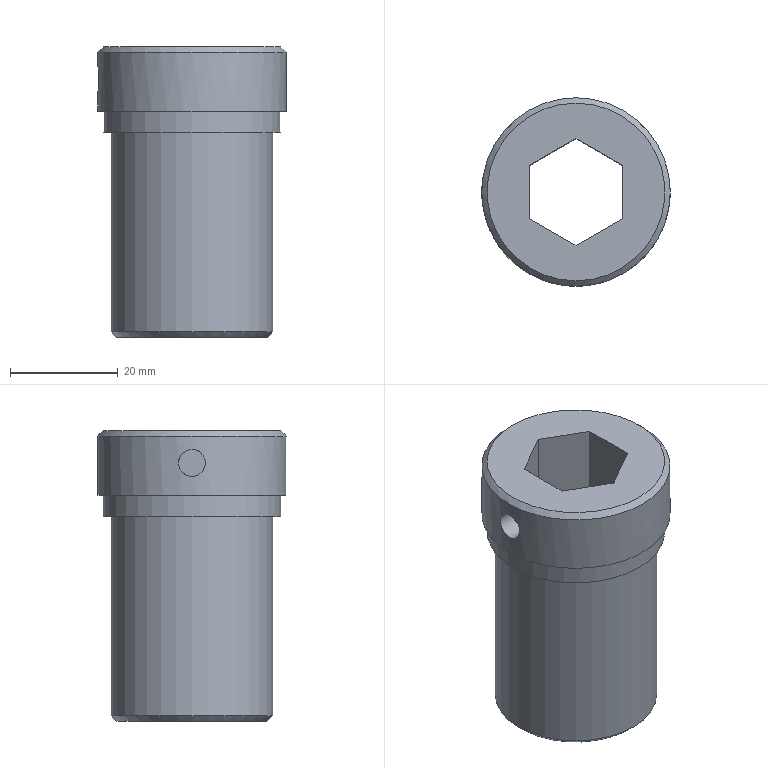Part | STEP file | JBJ-P-1002-08 | 1 solid | 16 faces | box 35 x 35 x 54 mm | volume 27719 mm3 | plane 10 | cylinder 4 | cone 2 | commonest cylinder face diameters 5 x1 30 x1 33 x1 35 x1
STEP:
#1=CARTESIAN_POINT('',(8.6,4.965,-54.));
#2=VERTEX_POINT('',#1);
#3=CARTESIAN_POINT('',(0.,9.93,-54.));
#4=VERTEX_POINT('',#3);
#5=CARTESIAN_POINT('',(8.6,4.965,-54.));
#6=DIRECTION('',(-0.866,0.5,0.));
#7=VECTOR('',#6,1000.);
#8=LINE('',#5,#7);
#9=EDGE_CURVE('',#2,#4,#8,.T.);
#10=ORIENTED_EDGE('',*,*,#9,.T.);
#11=CARTESIAN_POINT('',(-8.6,4.965,-54.));
#12=VERTEX_POINT('',#11);
#13=CARTESIAN_POINT('',(0.,9.93,-54.));
#14=DIRECTION('',(-0.866,-0.5,0.));
#15=VECTOR('',#14,1000.);
#16=LINE('',#13,#15);
#17=EDGE_CURVE('',#4,#12,#16,.T.);
#18=ORIENTED_EDGE('',*,*,#17,.T.);
#19=CARTESIAN_POINT('',(-8.6,-4.965,-54.));
#20=VERTEX_POINT('',#19);
#21=CARTESIAN_POINT('',(-8.6,4.965,-54.));
#22=DIRECTION('',(0.,-1.,0.));
#23=VECTOR('',#22,1000.);
#24=LINE('',#21,#23);
#25=EDGE_CURVE('',#12,#20,#24,.T.);
#26=ORIENTED_EDGE('',*,*,#25,.T.);
#27=CARTESIAN_POINT('',(0.,-9.93,-54.));
#28=VERTEX_POINT('',#27);
#29=CARTESIAN_POINT('',(-8.6,-4.965,-54.));
#30=DIRECTION('',(0.866,-0.5,0.));
#31=VECTOR('',#30,1000.);
#32=LINE('',#29,#31);
#33=EDGE_CURVE('',#20,#28,#32,.T.);
#34=ORIENTED_EDGE('',*,*,#33,.T.);
#35=CARTESIAN_POINT('',(8.6,-4.965,-54.));
#36=VERTEX_POINT('',#35);
#37=CARTESIAN_POINT('',(0.,-9.93,-54.));
#38=DIRECTION('',(0.866,0.5,0.));
#39=VECTOR('',#38,1000.);
#40=LINE('',#37,#39);
#41=EDGE_CURVE('',#28,#36,#40,.T.);
#42=ORIENTED_EDGE('',*,*,#41,.T.);
#43=CARTESIAN_POINT('',(8.6,-4.965,-54.));
#44=DIRECTION('',(0.,1.,0.));
#45=VECTOR('',#44,1000.);
#46=LINE('',#43,#45);
#47=EDGE_CURVE('',#36,#2,#46,.T.);
#48=ORIENTED_EDGE('',*,*,#47,.T.);
#49=EDGE_LOOP('',(#10,#18,#26,#34,#42,#48));
#50=FACE_BOUND('',#49,.T.);
#51=CARTESIAN_POINT('',(0.,14.,-54.));
#52=VERTEX_POINT('',#51);
#53=CARTESIAN_POINT('',(0.,0.,-54.));
#54=DIRECTION('',(0.,0.,-1.));
#55=DIRECTION('',(0.,1.,0.));
#56=AXIS2_PLACEMENT_3D('',#53,#54,#55);
#57=CIRCLE('',#56,14.);
#58=EDGE_CURVE('',#52,#52,#57,.T.);
#59=ORIENTED_EDGE('',*,*,#58,.T.);
#60=EDGE_LOOP('',(#59));
#61=FACE_OUTER_BOUND('',#60,.T.);
#62=CARTESIAN_POINT('',(0.,0.,-54.));
#63=DIRECTION('',(0.,0.,-1.));
#64=DIRECTION('',(0.,1.,0.));
#65=AXIS2_PLACEMENT_3D('',#62,#63,#64);
#66=PLANE('',#65);
#67=ADVANCED_FACE('',(#50,#61),#66,.T.);
#68=ORIENTED_EDGE('',*,*,#58,.F.);
#69=EDGE_LOOP('',(#68));
#70=FACE_BOUND('',#69,.T.);
#71=CARTESIAN_POINT('',(0.,15.,-53.));
#72=VERTEX_POINT('',#71);
#73=CARTESIAN_POINT('',(0.,0.,-53.));
#74=DIRECTION('',(0.,0.,-1.));
#75=DIRECTION('',(0.,1.,0.));
#76=AXIS2_PLACEMENT_3D('',#73,#74,#75);
#77=CIRCLE('',#76,15.);
#78=EDGE_CURVE('',#72,#72,#77,.T.);
#79=ORIENTED_EDGE('',*,*,#78,.T.);
#80=EDGE_LOOP('',(#79));
#81=FACE_OUTER_BOUND('',#80,.T.);
#82=CARTESIAN_POINT('',(0.,0.,-53.));
#83=DIRECTION('',(0.,0.,1.));
#84=DIRECTION('',(0.,-1.,0.));
#85=AXIS2_PLACEMENT_3D('',#82,#83,#84);
#86=CONICAL_SURFACE('',#85,15.,0.7854);
#87=ADVANCED_FACE('',(#70,#81),#86,.T.);
#88=ORIENTED_EDGE('',*,*,#78,.F.);
#89=EDGE_LOOP('',(#88));
#90=FACE_OUTER_BOUND('',#89,.T.);
#91=CARTESIAN_POINT('',(0.,15.,-16.));
#92=VERTEX_POINT('',#91);
#93=CARTESIAN_POINT('',(0.,0.,-16.));
#94=DIRECTION('',(0.,0.,-1.));
#95=DIRECTION('',(0.,1.,0.));
#96=AXIS2_PLACEMENT_3D('',#93,#94,#95);
#97=CIRCLE('',#96,15.);
#98=EDGE_CURVE('',#92,#92,#97,.T.);
#99=ORIENTED_EDGE('',*,*,#98,.T.);
#100=EDGE_LOOP('',(#99));
#101=FACE_OUTER_BOUND('',#100,.T.);
#102=CARTESIAN_POINT('',(0.,0.,-54.));
#103=DIRECTION('',(0.,0.,-1.));
#104=DIRECTION('',(0.,1.,0.));
#105=AXIS2_PLACEMENT_3D('',#102,#103,#104);
#106=CYLINDRICAL_SURFACE('',#105,15.);
#107=ADVANCED_FACE('',(#90,#101),#106,.T.);
#108=ORIENTED_EDGE('',*,*,#98,.F.);
#109=EDGE_LOOP('',(#108));
#110=FACE_BOUND('',#109,.T.);
#111=CARTESIAN_POINT('',(0.,16.5,-16.));
#112=VERTEX_POINT('',#111);
#113=CARTESIAN_POINT('',(0.,0.,-16.));
#114=DIRECTION('',(0.,0.,-1.));
#115=DIRECTION('',(0.,1.,0.));
#116=AXIS2_PLACEMENT_3D('',#113,#114,#115);
#117=CIRCLE('',#116,16.5);
#118=EDGE_CURVE('',#112,#112,#117,.T.);
#119=ORIENTED_EDGE('',*,*,#118,.T.);
#120=EDGE_LOOP('',(#119));
#121=FACE_OUTER_BOUND('',#120,.T.);
#122=CARTESIAN_POINT('',(0.,0.,-16.));
#123=DIRECTION('',(0.,0.,1.));
#124=DIRECTION('',(0.,-1.,0.));
#125=AXIS2_PLACEMENT_3D('',#122,#123,#124);
#126=PLANE('',#125);
#127=ADVANCED_FACE('',(#110,#121),#126,.F.);
#128=ORIENTED_EDGE('',*,*,#118,.F.);
#129=EDGE_LOOP('',(#128));
#130=FACE_OUTER_BOUND('',#129,.T.);
#131=CARTESIAN_POINT('',(0.,16.5,-12.));
#132=VERTEX_POINT('',#131);
#133=CARTESIAN_POINT('',(0.,0.,-12.));
#134=DIRECTION('',(0.,0.,-1.));
#135=DIRECTION('',(0.,1.,0.));
#136=AXIS2_PLACEMENT_3D('',#133,#134,#135);
#137=CIRCLE('',#136,16.5);
#138=EDGE_CURVE('',#132,#132,#137,.T.);
#139=ORIENTED_EDGE('',*,*,#138,.T.);
#140=EDGE_LOOP('',(#139));
#141=FACE_OUTER_BOUND('',#140,.T.);
#142=CARTESIAN_POINT('',(0.,0.,-54.));
#143=DIRECTION('',(0.,0.,-1.));
#144=DIRECTION('',(0.,1.,0.));
#145=AXIS2_PLACEMENT_3D('',#142,#143,#144);
#146=CYLINDRICAL_SURFACE('',#145,16.5);
#147=ADVANCED_FACE('',(#130,#141),#146,.T.);
#148=ORIENTED_EDGE('',*,*,#138,.F.);
#149=EDGE_LOOP('',(#148));
#150=FACE_BOUND('',#149,.T.);
#151=CARTESIAN_POINT('',(0.,17.5,-12.));
#152=VERTEX_POINT('',#151);
#153=CARTESIAN_POINT('',(0.,0.,-12.));
#154=DIRECTION('',(0.,0.,-1.));
#155=DIRECTION('',(0.,1.,0.));
#156=AXIS2_PLACEMENT_3D('',#153,#154,#155);
#157=CIRCLE('',#156,17.5);
#158=EDGE_CURVE('',#152,#152,#157,.T.);
#159=ORIENTED_EDGE('',*,*,#158,.T.);
#160=EDGE_LOOP('',(#159));
#161=FACE_OUTER_BOUND('',#160,.T.);
#162=CARTESIAN_POINT('',(0.,0.,-12.));
#163=DIRECTION('',(0.,0.,1.));
#164=DIRECTION('',(0.,-1.,0.));
#165=AXIS2_PLACEMENT_3D('',#162,#163,#164);
#166=PLANE('',#165);
#167=ADVANCED_FACE('',(#150,#161),#166,.F.);
#168=CARTESIAN_POINT('',(0.,-17.5,-1.));
#169=VERTEX_POINT('',#168);
#170=CARTESIAN_POINT('',(0.,0.,-1.));
#171=DIRECTION('',(0.,0.,-1.));
#172=DIRECTION('',(0.,-1.,0.));
#173=AXIS2_PLACEMENT_3D('',#170,#171,#172);
#174=CIRCLE('',#173,17.5);
#175=EDGE_CURVE('',#169,#169,#174,.T.);
#176=ORIENTED_EDGE('',*,*,#175,.T.);
#177=EDGE_LOOP('',(#176));
#178=FACE_OUTER_BOUND('',#177,.T.);
#179=CARTESIAN_POINT('',(-17.5,0.,-3.5));
#180=VERTEX_POINT('',#179);
#181=CARTESIAN_POINT('',(-17.5,0.,-3.5));
#182=CARTESIAN_POINT('',(-17.5,-0.1654,-3.5));
#183=CARTESIAN_POINT('',(-17.498,-0.328,-3.516));
#184=CARTESIAN_POINT('',(-17.489,-0.6478,-3.58));
#185=CARTESIAN_POINT('',(-17.482,-0.8067,-3.628));
#186=CARTESIAN_POINT('',(-17.465,-1.109,-3.754));
#187=CARTESIAN_POINT('',(-17.456,-1.253,-3.83));
#188=CARTESIAN_POINT('',(-17.434,-1.524,-4.012));
#189=CARTESIAN_POINT('',(-17.422,-1.653,-4.117));
#190=CARTESIAN_POINT('',(-17.399,-1.883,-4.348));
#191=CARTESIAN_POINT('',(-17.387,-1.987,-4.473));
#192=CARTESIAN_POINT('',(-17.365,-2.169,-4.747));
#193=CARTESIAN_POINT('',(-17.355,-2.247,-4.892));
#194=CARTESIAN_POINT('',(-17.339,-2.372,-5.192));
#195=CARTESIAN_POINT('',(-17.332,-2.42,-5.35));
#196=CARTESIAN_POINT('',(-17.323,-2.484,-5.673));
#197=CARTESIAN_POINT('',(-17.321,-2.5,-5.835));
#198=CARTESIAN_POINT('',(-17.32,-2.5,-6.162));
#199=CARTESIAN_POINT('',(-17.323,-2.484,-6.328));
#200=CARTESIAN_POINT('',(-17.332,-2.42,-6.649));
#201=CARTESIAN_POINT('',(-17.339,-2.373,-6.804));
#202=CARTESIAN_POINT('',(-17.355,-2.247,-7.107));
#203=CARTESIAN_POINT('',(-17.365,-2.169,-7.253));
#204=CARTESIAN_POINT('',(-17.387,-1.988,-7.524));
#205=CARTESIAN_POINT('',(-17.399,-1.885,-7.651));
#206=CARTESIAN_POINT('',(-17.422,-1.652,-7.884));
#207=CARTESIAN_POINT('',(-17.434,-1.526,-7.987));
#208=CARTESIAN_POINT('',(-17.455,-1.255,-8.168));
#209=CARTESIAN_POINT('',(-17.465,-1.109,-8.246));
#210=CARTESIAN_POINT('',(-17.482,-0.8066,-8.372));
#211=CARTESIAN_POINT('',(-17.489,-0.6508,-8.419));
#212=CARTESIAN_POINT('',(-17.498,-0.33,-8.484));
#213=CARTESIAN_POINT('',(-17.5,-0.1642,-8.5));
#214=CARTESIAN_POINT('',(-17.5,0.1623,-8.5));
#215=CARTESIAN_POINT('',(-17.498,0.3247,-8.484));
#216=CARTESIAN_POINT('',(-17.489,0.6478,-8.42));
#217=CARTESIAN_POINT('',(-17.482,0.8054,-8.372));
#218=CARTESIAN_POINT('',(-17.466,1.106,-8.248));
#219=CARTESIAN_POINT('',(-17.456,1.252,-8.17));
#220=CARTESIAN_POINT('',(-17.434,1.525,-7.988));
#221=CARTESIAN_POINT('',(-17.422,1.651,-7.885));
#222=CARTESIAN_POINT('',(-17.399,1.881,-7.654));
#223=CARTESIAN_POINT('',(-17.387,1.987,-7.526));
#224=CARTESIAN_POINT('',(-17.365,2.168,-7.255));
#225=CARTESIAN_POINT('',(-17.355,2.245,-7.111));
#226=CARTESIAN_POINT('',(-17.339,2.371,-6.809));
#227=CARTESIAN_POINT('',(-17.332,2.42,-6.65));
#228=CARTESIAN_POINT('',(-17.323,2.483,-6.33));
#229=CARTESIAN_POINT('',(-17.321,2.5,-6.167));
#230=CARTESIAN_POINT('',(-17.32,2.5,-5.837));
#231=CARTESIAN_POINT('',(-17.323,2.484,-5.674));
#232=CARTESIAN_POINT('',(-17.332,2.421,-5.354));
#233=CARTESIAN_POINT('',(-17.339,2.373,-5.195));
#234=CARTESIAN_POINT('',(-17.355,2.247,-4.893));
#235=CARTESIAN_POINT('',(-17.365,2.171,-4.749));
#236=CARTESIAN_POINT('',(-17.387,1.989,-4.477));
#237=CARTESIAN_POINT('',(-17.399,1.884,-4.349));
#238=CARTESIAN_POINT('',(-17.434,1.539,-4.003));
#239=CARTESIAN_POINT('',(-17.457,1.261,-3.817));
#240=CARTESIAN_POINT('',(-17.482,0.8097,-3.629));
#241=CARTESIAN_POINT('',(-17.489,0.6519,-3.581));
#242=CARTESIAN_POINT('',(-17.498,0.3288,-3.516));
#243=CARTESIAN_POINT('',(-17.5,0.1654,-3.5));
#244=CARTESIAN_POINT('',(-17.5,0.,-3.5));
#245=B_SPLINE_CURVE_WITH_KNOTS('',3,(#181,#182,#183,#184,#185,#186,#187,#188,#189,#190,#191,#192,#193,#194,#195,#196,#197,#198,#199,#200,#201,#202,#203,#204,#205,#206,#207,#208,#209,#210,#211,#212,#213,#214,#215,#216,#217,#218,#219,#220,#221,#222,#223,#224,#225,#226,#227,#228,#229,#230,#231,#232,#233,#234,#235,#236,#237,#238,#239,#240,#241,#242,#243,#244),.UNSPECIFIED.,.T.,.F.,(4,2,2,2,2,2,2,2,2,2,2,2,2,2,2,2,2,2,2,2,2,2,2,2,2,2,2,2,2,2,2,4),(0.,0.0004891,0.0009781,0.001467,0.001956,0.002445,0.002934,0.003424,0.003913,0.004402,0.004891,0.00538,0.005869,0.006358,0.006847,0.007336,0.007825,0.008314,0.008803,0.009292,0.009781,0.01027,0.01076,0.01125,0.01174,0.01223,0.01272,0.01321,0.01369,0.01467,0.01516,0.01565),.UNSPECIFIED.);
#246=EDGE_CURVE('',#180,#180,#245,.T.);
#247=ORIENTED_EDGE('',*,*,#246,.T.);
#248=EDGE_LOOP('',(#247));
#249=FACE_BOUND('',#248,.T.);
#250=ORIENTED_EDGE('',*,*,#158,.F.);
#251=EDGE_LOOP('',(#250));
#252=FACE_OUTER_BOUND('',#251,.T.);
#253=CARTESIAN_POINT('',(0.,0.,-54.));
#254=DIRECTION('',(0.,0.,-1.));
#255=DIRECTION('',(0.,1.,0.));
#256=AXIS2_PLACEMENT_3D('',#253,#254,#255);
#257=CYLINDRICAL_SURFACE('',#256,17.5);
#258=ADVANCED_FACE('',(#178,#249,#252),#257,.T.);
#259=CARTESIAN_POINT('',(0.,-16.5,0.));
#260=VERTEX_POINT('',#259);
#261=CARTESIAN_POINT('',(0.,0.,0.));
#262=DIRECTION('',(0.,0.,1.));
#263=DIRECTION('',(0.,-1.,0.));
#264=AXIS2_PLACEMENT_3D('',#261,#262,#263);
#265=CIRCLE('',#264,16.5);
#266=EDGE_CURVE('',#260,#260,#265,.T.);
#267=ORIENTED_EDGE('',*,*,#266,.T.);
#268=EDGE_LOOP('',(#267));
#269=FACE_OUTER_BOUND('',#268,.T.);
#270=CARTESIAN_POINT('',(8.6,4.965,0.));
#271=VERTEX_POINT('',#270);
#272=CARTESIAN_POINT('',(0.,9.93,0.));
#273=VERTEX_POINT('',#272);
#274=CARTESIAN_POINT('',(8.6,4.965,0.));
#275=DIRECTION('',(-0.866,0.5,0.));
#276=VECTOR('',#275,1000.);
#277=LINE('',#274,#276);
#278=EDGE_CURVE('',#271,#273,#277,.T.);
#279=ORIENTED_EDGE('',*,*,#278,.F.);
#280=CARTESIAN_POINT('',(8.6,-4.965,0.));
#281=VERTEX_POINT('',#280);
#282=CARTESIAN_POINT('',(8.6,-4.965,0.));
#283=DIRECTION('',(0.,1.,0.));
#284=VECTOR('',#283,1000.);
#285=LINE('',#282,#284);
#286=EDGE_CURVE('',#281,#271,#285,.T.);
#287=ORIENTED_EDGE('',*,*,#286,.F.);
#288=CARTESIAN_POINT('',(0.,-9.93,0.));
#289=VERTEX_POINT('',#288);
#290=CARTESIAN_POINT('',(0.,-9.93,0.));
#291=DIRECTION('',(0.866,0.5,0.));
#292=VECTOR('',#291,1000.);
#293=LINE('',#290,#292);
#294=EDGE_CURVE('',#289,#281,#293,.T.);
#295=ORIENTED_EDGE('',*,*,#294,.F.);
#296=CARTESIAN_POINT('',(-8.6,-4.965,0.));
#297=VERTEX_POINT('',#296);
#298=CARTESIAN_POINT('',(-8.6,-4.965,0.));
#299=DIRECTION('',(0.866,-0.5,0.));
#300=VECTOR('',#299,1000.);
#301=LINE('',#298,#300);
#302=EDGE_CURVE('',#297,#289,#301,.T.);
#303=ORIENTED_EDGE('',*,*,#302,.F.);
#304=CARTESIAN_POINT('',(-8.6,4.965,0.));
#305=VERTEX_POINT('',#304);
#306=CARTESIAN_POINT('',(-8.6,4.965,0.));
#307=DIRECTION('',(0.,-1.,0.));
#308=VECTOR('',#307,1000.);
#309=LINE('',#306,#308);
#310=EDGE_CURVE('',#305,#297,#309,.T.);
#311=ORIENTED_EDGE('',*,*,#310,.F.);
#312=CARTESIAN_POINT('',(0.,9.93,0.));
#313=DIRECTION('',(-0.866,-0.5,0.));
#314=VECTOR('',#313,1000.);
#315=LINE('',#312,#314);
#316=EDGE_CURVE('',#273,#305,#315,.T.);
#317=ORIENTED_EDGE('',*,*,#316,.F.);
#318=EDGE_LOOP('',(#279,#287,#295,#303,#311,#317));
#319=FACE_BOUND('',#318,.T.);
#320=CARTESIAN_POINT('',(0.,0.,0.));
#321=DIRECTION('',(0.,0.,1.));
#322=DIRECTION('',(0.,-1.,0.));
#323=AXIS2_PLACEMENT_3D('',#320,#321,#322);
#324=PLANE('',#323);
#325=ADVANCED_FACE('',(#269,#319),#324,.T.);
#326=ORIENTED_EDGE('',*,*,#278,.T.);
#327=CARTESIAN_POINT('',(0.,9.93,-54.));
#328=DIRECTION('',(0.,0.,1.));
#329=VECTOR('',#328,1000.);
#330=LINE('',#327,#329);
#331=EDGE_CURVE('',#4,#273,#330,.T.);
#332=ORIENTED_EDGE('',*,*,#331,.F.);
#333=ORIENTED_EDGE('',*,*,#9,.F.);
#334=CARTESIAN_POINT('',(8.6,4.965,-54.));
#335=DIRECTION('',(0.,0.,1.));
#336=VECTOR('',#335,1000.);
#337=LINE('',#334,#336);
#338=EDGE_CURVE('',#2,#271,#337,.T.);
#339=ORIENTED_EDGE('',*,*,#338,.T.);
#340=EDGE_LOOP('',(#326,#332,#333,#339));
#341=FACE_OUTER_BOUND('',#340,.T.);
#342=CARTESIAN_POINT('',(8.6,4.965,-54.));
#343=DIRECTION('',(0.5,0.866,0.));
#344=DIRECTION('',(-0.866,0.5,0.));
#345=AXIS2_PLACEMENT_3D('',#342,#343,#344);
#346=PLANE('',#345);
#347=ADVANCED_FACE('',(#341),#346,.F.);
#348=ORIENTED_EDGE('',*,*,#286,.T.);
#349=ORIENTED_EDGE('',*,*,#338,.F.);
#350=ORIENTED_EDGE('',*,*,#47,.F.);
#351=CARTESIAN_POINT('',(8.6,-4.965,-54.));
#352=DIRECTION('',(0.,0.,1.));
#353=VECTOR('',#352,1000.);
#354=LINE('',#351,#353);
#355=EDGE_CURVE('',#36,#281,#354,.T.);
#356=ORIENTED_EDGE('',*,*,#355,.T.);
#357=EDGE_LOOP('',(#348,#349,#350,#356));
#358=FACE_OUTER_BOUND('',#357,.T.);
#359=CARTESIAN_POINT('',(8.6,-4.965,-54.));
#360=DIRECTION('',(1.,0.,0.));
#361=DIRECTION('',(0.,1.,0.));
#362=AXIS2_PLACEMENT_3D('',#359,#360,#361);
#363=PLANE('',#362);
#364=ADVANCED_FACE('',(#358),#363,.F.);
#365=ORIENTED_EDGE('',*,*,#294,.T.);
#366=ORIENTED_EDGE('',*,*,#355,.F.);
#367=ORIENTED_EDGE('',*,*,#41,.F.);
#368=CARTESIAN_POINT('',(0.,-9.93,-54.));
#369=DIRECTION('',(0.,0.,1.));
#370=VECTOR('',#369,1000.);
#371=LINE('',#368,#370);
#372=EDGE_CURVE('',#28,#289,#371,.T.);
#373=ORIENTED_EDGE('',*,*,#372,.T.);
#374=EDGE_LOOP('',(#365,#366,#367,#373));
#375=FACE_OUTER_BOUND('',#374,.T.);
#376=CARTESIAN_POINT('',(0.,-9.93,-54.));
#377=DIRECTION('',(0.5,-0.866,0.));
#378=DIRECTION('',(0.866,0.5,0.));
#379=AXIS2_PLACEMENT_3D('',#376,#377,#378);
#380=PLANE('',#379);
#381=ADVANCED_FACE('',(#375),#380,.F.);
#382=ORIENTED_EDGE('',*,*,#302,.T.);
#383=ORIENTED_EDGE('',*,*,#372,.F.);
#384=ORIENTED_EDGE('',*,*,#33,.F.);
#385=CARTESIAN_POINT('',(-8.6,-4.965,-54.));
#386=DIRECTION('',(0.,0.,1.));
#387=VECTOR('',#386,1000.);
#388=LINE('',#385,#387);
#389=EDGE_CURVE('',#20,#297,#388,.T.);
#390=ORIENTED_EDGE('',*,*,#389,.T.);
#391=EDGE_LOOP('',(#382,#383,#384,#390));
#392=FACE_OUTER_BOUND('',#391,.T.);
#393=CARTESIAN_POINT('',(-8.6,-4.965,-54.));
#394=DIRECTION('',(-0.5,-0.866,0.));
#395=DIRECTION('',(0.866,-0.5,0.));
#396=AXIS2_PLACEMENT_3D('',#393,#394,#395);
#397=PLANE('',#396);
#398=ADVANCED_FACE('',(#392),#397,.F.);
#399=CARTESIAN_POINT('',(-8.6,0.,-3.5));
#400=VERTEX_POINT('',#399);
#401=CARTESIAN_POINT('',(-8.6,0.,-6.));
#402=DIRECTION('',(-1.,0.,0.));
#403=DIRECTION('',(0.,0.,1.));
#404=AXIS2_PLACEMENT_3D('',#401,#402,#403);
#405=CIRCLE('',#404,2.5);
#406=EDGE_CURVE('',#400,#400,#405,.T.);
#407=ORIENTED_EDGE('',*,*,#406,.T.);
#408=EDGE_LOOP('',(#407));
#409=FACE_BOUND('',#408,.T.);
#410=ORIENTED_EDGE('',*,*,#310,.T.);
#411=ORIENTED_EDGE('',*,*,#389,.F.);
#412=ORIENTED_EDGE('',*,*,#25,.F.);
#413=CARTESIAN_POINT('',(-8.6,4.965,-54.));
#414=DIRECTION('',(0.,0.,1.));
#415=VECTOR('',#414,1000.);
#416=LINE('',#413,#415);
#417=EDGE_CURVE('',#12,#305,#416,.T.);
#418=ORIENTED_EDGE('',*,*,#417,.T.);
#419=EDGE_LOOP('',(#410,#411,#412,#418));
#420=FACE_OUTER_BOUND('',#419,.T.);
#421=CARTESIAN_POINT('',(-8.6,4.965,-54.));
#422=DIRECTION('',(-1.,0.,0.));
#423=DIRECTION('',(0.,0.,1.));
#424=AXIS2_PLACEMENT_3D('',#421,#422,#423);
#425=PLANE('',#424);
#426=ADVANCED_FACE('',(#409,#420),#425,.F.);
#427=ORIENTED_EDGE('',*,*,#316,.T.);
#428=ORIENTED_EDGE('',*,*,#417,.F.);
#429=ORIENTED_EDGE('',*,*,#17,.F.);
#430=ORIENTED_EDGE('',*,*,#331,.T.);
#431=EDGE_LOOP('',(#427,#428,#429,#430));
#432=FACE_OUTER_BOUND('',#431,.T.);
#433=CARTESIAN_POINT('',(0.,9.93,-54.));
#434=DIRECTION('',(-0.5,0.866,0.));
#435=DIRECTION('',(-0.866,-0.5,0.));
#436=AXIS2_PLACEMENT_3D('',#433,#434,#435);
#437=PLANE('',#436);
#438=ADVANCED_FACE('',(#432),#437,.F.);
#439=ORIENTED_EDGE('',*,*,#406,.F.);
#440=EDGE_LOOP('',(#439));
#441=FACE_OUTER_BOUND('',#440,.T.);
#442=ORIENTED_EDGE('',*,*,#246,.F.);
#443=EDGE_LOOP('',(#442));
#444=FACE_OUTER_BOUND('',#443,.T.);
#445=CARTESIAN_POINT('',(-17.5,0.,-6.));
#446=DIRECTION('',(-1.,0.,0.));
#447=DIRECTION('',(0.,0.,1.));
#448=AXIS2_PLACEMENT_3D('',#445,#446,#447);
#449=CYLINDRICAL_SURFACE('',#448,2.5);
#450=ADVANCED_FACE('',(#441,#444),#449,.F.);
#451=ORIENTED_EDGE('',*,*,#266,.F.);
#452=EDGE_LOOP('',(#451));
#453=FACE_BOUND('',#452,.T.);
#454=ORIENTED_EDGE('',*,*,#175,.F.);
#455=EDGE_LOOP('',(#454));
#456=FACE_OUTER_BOUND('',#455,.T.);
#457=CARTESIAN_POINT('',(0.,0.,-1.));
#458=DIRECTION('',(0.,0.,-1.));
#459=DIRECTION('',(0.,1.,0.));
#460=AXIS2_PLACEMENT_3D('',#457,#458,#459);
#461=CONICAL_SURFACE('',#460,17.5,0.7854);
#462=ADVANCED_FACE('',(#453,#456),#461,.T.);
#463=CLOSED_SHELL('',(#67,#87,#107,#127,#147,#167,#258,#325,#347,#364,#381,#398,#426,#438,#450,#462));
#464=MANIFOLD_SOLID_BREP('',#463);
#465=CARTESIAN_POINT('',(0.,0.,0.));
#466=DIRECTION('',(0.,0.,1.));
#467=DIRECTION('',(1.,0.,0.));
#468=AXIS2_PLACEMENT_3D('',#465,#466,#467);
#469=(LENGTH_UNIT()NAMED_UNIT(*)SI_UNIT(.MILLI.,.METRE.));
#470=UNCERTAINTY_MEASURE_WITH_UNIT(LENGTH_MEASURE(0.00001),#469,'','');
#471=(NAMED_UNIT(*)PLANE_ANGLE_UNIT()SI_UNIT($,.RADIAN.));
#472=(NAMED_UNIT(*)SI_UNIT($,.STERADIAN.)SOLID_ANGLE_UNIT());
#473=(GEOMETRIC_REPRESENTATION_CONTEXT(3)GLOBAL_UNCERTAINTY_ASSIGNED_CONTEXT((#470))GLOBAL_UNIT_ASSIGNED_CONTEXT((#469,#471,#472))REPRESENTATION_CONTEXT('',''));
#474=ADVANCED_BREP_SHAPE_REPRESENTATION('',(#464,#468),#473);